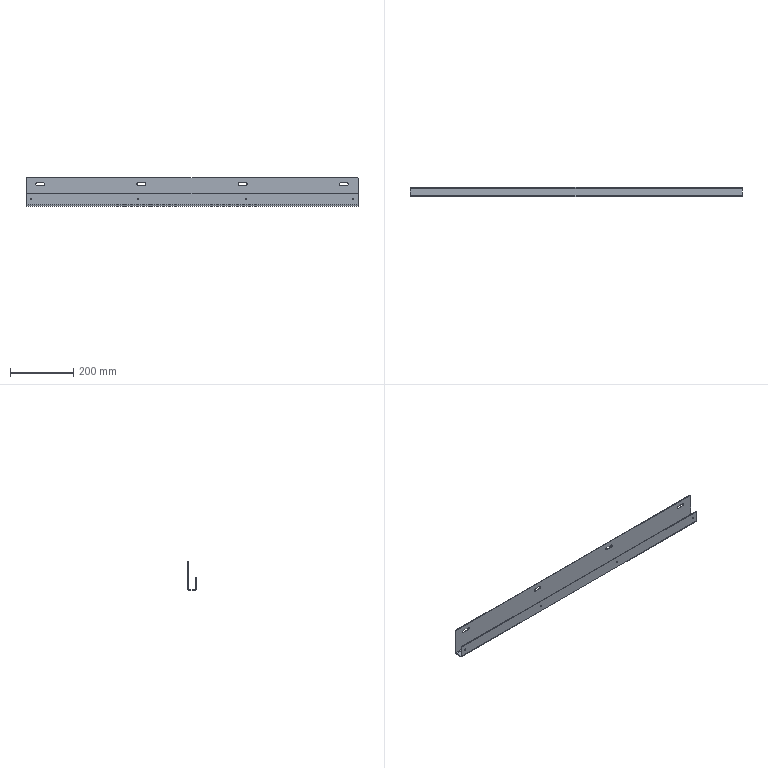Part | NX | features BREP 1 | 1 solid | 50 faces | box 1050 x 28.5 x 90 mm | volume 317181 mm3 | plane 30 | cylinder 20 | commonest cylinder face diameters 4.2 x8 8.2 x8 4 x2 8 x2
STEP:
#1=CARTESIAN_POINT('',(525.,-28.5,-52.));
#2=VERTEX_POINT('',#1);
#3=CARTESIAN_POINT('',(523.,-28.5,-50.));
#4=VERTEX_POINT('',#3);
#5=CARTESIAN_POINT('',(523.,-28.5,-50.));
#6=DIRECTION('',(-0.7071,0.,0.7071));
#7=VECTOR('',#6,1000.);
#8=LINE('',#5,#7);
#9=EDGE_CURVE('',#2,#4,#8,.T.);
#10=ORIENTED_EDGE('',*,*,#9,.F.);
#11=CARTESIAN_POINT('',(525.,-26.5,-52.));
#12=VERTEX_POINT('',#11);
#13=CARTESIAN_POINT('',(525.,-24.5,-52.));
#14=DIRECTION('',(0.,-1.,0.));
#15=VECTOR('',#14,1000.);
#16=LINE('',#13,#15);
#17=EDGE_CURVE('',#12,#2,#16,.T.);
#18=ORIENTED_EDGE('',*,*,#17,.F.);
#19=CARTESIAN_POINT('',(523.,-26.5,-50.));
#20=VERTEX_POINT('',#19);
#21=CARTESIAN_POINT('',(544.,-26.5,-71.));
#22=DIRECTION('',(0.7071,0.,-0.7071));
#23=VECTOR('',#22,1000.);
#24=LINE('',#21,#23);
#25=EDGE_CURVE('',#20,#12,#24,.T.);
#26=ORIENTED_EDGE('',*,*,#25,.F.);
#27=CARTESIAN_POINT('',(523.,-28.5,-50.));
#28=DIRECTION('',(0.,1.,0.));
#29=VECTOR('',#28,1000.);
#30=LINE('',#27,#29);
#31=EDGE_CURVE('',#4,#20,#30,.T.);
#32=ORIENTED_EDGE('',*,*,#31,.F.);
#33=EDGE_LOOP('',(#10,#18,#26,#32));
#34=FACE_BOUND('',#33,.T.);
#35=CARTESIAN_POINT('',(523.,-28.5,-50.));
#36=DIRECTION('',(-0.7071,0.,-0.7071));
#37=DIRECTION('',(0.,1.,0.));
#38=AXIS2_PLACEMENT_3D('',#35,#36,#37);
#39=PLANE('',#38);
#40=ADVANCED_FACE('',(#34),#39,.F.);
#41=CARTESIAN_POINT('',(525.,-2.,-2.));
#42=VERTEX_POINT('',#41);
#43=CARTESIAN_POINT('',(523.,-2.,0.));
#44=VERTEX_POINT('',#43);
#45=CARTESIAN_POINT('',(569.,-2.,-46.));
#46=DIRECTION('',(-0.7071,0.,0.7071));
#47=VECTOR('',#46,1000.);
#48=LINE('',#45,#47);
#49=EDGE_CURVE('',#42,#44,#48,.T.);
#50=ORIENTED_EDGE('',*,*,#49,.F.);
#51=CARTESIAN_POINT('',(525.,0.,-2.));
#52=VERTEX_POINT('',#51);
#53=CARTESIAN_POINT('',(525.,-4.,-2.));
#54=DIRECTION('',(0.,-1.,0.));
#55=VECTOR('',#54,1000.);
#56=LINE('',#53,#55);
#57=EDGE_CURVE('',#52,#42,#56,.T.);
#58=ORIENTED_EDGE('',*,*,#57,.F.);
#59=CARTESIAN_POINT('',(523.,0.,0.));
#60=VERTEX_POINT('',#59);
#61=CARTESIAN_POINT('',(523.,0.,0.));
#62=DIRECTION('',(0.7071,0.,-0.7071));
#63=VECTOR('',#62,1000.);
#64=LINE('',#61,#63);
#65=EDGE_CURVE('',#60,#52,#64,.T.);
#66=ORIENTED_EDGE('',*,*,#65,.F.);
#67=CARTESIAN_POINT('',(523.,-2.,0.));
#68=DIRECTION('',(0.,1.,0.));
#69=VECTOR('',#68,1000.);
#70=LINE('',#67,#69);
#71=EDGE_CURVE('',#44,#60,#70,.T.);
#72=ORIENTED_EDGE('',*,*,#71,.F.);
#73=EDGE_LOOP('',(#50,#58,#66,#72));
#74=FACE_BOUND('',#73,.T.);
#75=CARTESIAN_POINT('',(523.,-2.,0.));
#76=DIRECTION('',(-0.7071,0.,-0.7071));
#77=DIRECTION('',(0.,1.,0.));
#78=AXIS2_PLACEMENT_3D('',#75,#76,#77);
#79=PLANE('',#78);
#80=ADVANCED_FACE('',(#74),#79,.F.);
#81=CARTESIAN_POINT('',(-523.,-28.5,-50.));
#82=VERTEX_POINT('',#81);
#83=CARTESIAN_POINT('',(-525.,-28.5,-52.));
#84=VERTEX_POINT('',#83);
#85=CARTESIAN_POINT('',(-525.,-28.5,-52.));
#86=DIRECTION('',(-0.7071,0.,-0.7071));
#87=VECTOR('',#86,1000.);
#88=LINE('',#85,#87);
#89=EDGE_CURVE('',#82,#84,#88,.T.);
#90=ORIENTED_EDGE('',*,*,#89,.F.);
#91=CARTESIAN_POINT('',(-523.,-26.5,-50.));
#92=VERTEX_POINT('',#91);
#93=CARTESIAN_POINT('',(-523.,-28.5,-50.));
#94=DIRECTION('',(0.,-1.,0.));
#95=VECTOR('',#94,1000.);
#96=LINE('',#93,#95);
#97=EDGE_CURVE('',#92,#82,#96,.T.);
#98=ORIENTED_EDGE('',*,*,#97,.F.);
#99=CARTESIAN_POINT('',(-525.,-26.5,-52.));
#100=VERTEX_POINT('',#99);
#101=CARTESIAN_POINT('',(-19.,-26.5,454.));
#102=DIRECTION('',(0.7071,0.,0.7071));
#103=VECTOR('',#102,1000.);
#104=LINE('',#101,#103);
#105=EDGE_CURVE('',#100,#92,#104,.T.);
#106=ORIENTED_EDGE('',*,*,#105,.F.);
#107=CARTESIAN_POINT('',(-525.,-26.5,-52.));
#108=DIRECTION('',(0.,1.,0.));
#109=VECTOR('',#108,1000.);
#110=LINE('',#107,#109);
#111=EDGE_CURVE('',#84,#100,#110,.T.);
#112=ORIENTED_EDGE('',*,*,#111,.F.);
#113=EDGE_LOOP('',(#90,#98,#106,#112));
#114=FACE_BOUND('',#113,.T.);
#115=CARTESIAN_POINT('',(-525.,-4.,-52.));
#116=DIRECTION('',(-0.7071,0.,0.7071));
#117=DIRECTION('',(0.,-1.,0.));
#118=AXIS2_PLACEMENT_3D('',#115,#116,#117);
#119=PLANE('',#118);
#120=ADVANCED_FACE('',(#114),#119,.T.);
#121=CARTESIAN_POINT('',(-523.,-2.,0.));
#122=VERTEX_POINT('',#121);
#123=CARTESIAN_POINT('',(-525.,-2.,-2.));
#124=VERTEX_POINT('',#123);
#125=CARTESIAN_POINT('',(-44.,-2.,479.));
#126=DIRECTION('',(-0.7071,0.,-0.7071));
#127=VECTOR('',#126,1000.);
#128=LINE('',#125,#127);
#129=EDGE_CURVE('',#122,#124,#128,.T.);
#130=ORIENTED_EDGE('',*,*,#129,.F.);
#131=CARTESIAN_POINT('',(-523.,0.,0.));
#132=VERTEX_POINT('',#131);
#133=CARTESIAN_POINT('',(-523.,-2.,0.));
#134=DIRECTION('',(0.,-1.,0.));
#135=VECTOR('',#134,1000.);
#136=LINE('',#133,#135);
#137=EDGE_CURVE('',#132,#122,#136,.T.);
#138=ORIENTED_EDGE('',*,*,#137,.F.);
#139=CARTESIAN_POINT('',(-525.,0.,-2.));
#140=VERTEX_POINT('',#139);
#141=CARTESIAN_POINT('',(-525.,0.,-2.));
#142=DIRECTION('',(0.7071,0.,0.7071));
#143=VECTOR('',#142,1000.);
#144=LINE('',#141,#143);
#145=EDGE_CURVE('',#140,#132,#144,.T.);
#146=ORIENTED_EDGE('',*,*,#145,.F.);
#147=CARTESIAN_POINT('',(-525.,-4.,-2.));
#148=DIRECTION('',(0.,1.,0.));
#149=VECTOR('',#148,1000.);
#150=LINE('',#147,#149);
#151=EDGE_CURVE('',#124,#140,#150,.T.);
#152=ORIENTED_EDGE('',*,*,#151,.F.);
#153=EDGE_LOOP('',(#130,#138,#146,#152));
#154=FACE_BOUND('',#153,.T.);
#155=CARTESIAN_POINT('',(-525.,-4.,-2.));
#156=DIRECTION('',(0.7071,0.,-0.7071));
#157=DIRECTION('',(0.,1.,0.));
#158=AXIS2_PLACEMENT_3D('',#155,#156,#157);
#159=PLANE('',#158);
#160=ADVANCED_FACE('',(#154),#159,.F.);
#161=CARTESIAN_POINT('',(510.,-26.5,-65.9));
#162=VERTEX_POINT('',#161);
#163=CARTESIAN_POINT('',(510.,-28.5,-65.9));
#164=VERTEX_POINT('',#163);
#165=CARTESIAN_POINT('',(510.,-28.5,-65.9));
#166=DIRECTION('',(0.,-1.,0.));
#167=VECTOR('',#166,1000.);
#168=LINE('',#165,#167);
#169=EDGE_CURVE('',#162,#164,#168,.T.);
#170=ORIENTED_EDGE('',*,*,#169,.F.);
#171=CARTESIAN_POINT('',(510.,-26.5,-70.1));
#172=VERTEX_POINT('',#171);
#173=CARTESIAN_POINT('',(510.,-26.5,-68.));
#174=DIRECTION('',(0.,1.,0.));
#175=DIRECTION('',(0.,0.,1.));
#176=AXIS2_PLACEMENT_3D('',#173,#174,#175);
#177=CIRCLE('',#176,2.1);
#178=EDGE_CURVE('',#162,#172,#177,.T.);
#179=ORIENTED_EDGE('',*,*,#178,.T.);
#180=CARTESIAN_POINT('',(510.,-28.5,-70.1));
#181=VERTEX_POINT('',#180);
#182=CARTESIAN_POINT('',(510.,-28.5,-70.1));
#183=DIRECTION('',(0.,-1.,0.));
#184=VECTOR('',#183,1000.);
#185=LINE('',#182,#184);
#186=EDGE_CURVE('',#172,#181,#185,.T.);
#187=ORIENTED_EDGE('',*,*,#186,.T.);
#188=CARTESIAN_POINT('',(510.,-28.5,-68.));
#189=DIRECTION('',(0.,-1.,0.));
#190=DIRECTION('',(0.,0.,-1.));
#191=AXIS2_PLACEMENT_3D('',#188,#189,#190);
#192=CIRCLE('',#191,2.1);
#193=EDGE_CURVE('',#181,#164,#192,.T.);
#194=ORIENTED_EDGE('',*,*,#193,.T.);
#195=EDGE_LOOP('',(#170,#179,#187,#194));
#196=FACE_BOUND('',#195,.T.);
#197=CARTESIAN_POINT('',(510.,-28.5,-68.));
#198=DIRECTION('',(0.,-1.,0.));
#199=DIRECTION('',(0.,0.,-1.));
#200=AXIS2_PLACEMENT_3D('',#197,#198,#199);
#201=CYLINDRICAL_SURFACE('',#200,2.1);
#202=ADVANCED_FACE('',(#196),#201,.F.);
#203=CARTESIAN_POINT('',(170.,-26.5,-65.9));
#204=VERTEX_POINT('',#203);
#205=CARTESIAN_POINT('',(170.,-28.5,-65.9));
#206=VERTEX_POINT('',#205);
#207=CARTESIAN_POINT('',(170.,-28.5,-65.9));
#208=DIRECTION('',(0.,-1.,0.));
#209=VECTOR('',#208,1000.);
#210=LINE('',#207,#209);
#211=EDGE_CURVE('',#204,#206,#210,.T.);
#212=ORIENTED_EDGE('',*,*,#211,.F.);
#213=CARTESIAN_POINT('',(170.,-26.5,-70.1));
#214=VERTEX_POINT('',#213);
#215=CARTESIAN_POINT('',(170.,-26.5,-68.));
#216=DIRECTION('',(0.,1.,0.));
#217=DIRECTION('',(0.,0.,1.));
#218=AXIS2_PLACEMENT_3D('',#215,#216,#217);
#219=CIRCLE('',#218,2.1);
#220=EDGE_CURVE('',#204,#214,#219,.T.);
#221=ORIENTED_EDGE('',*,*,#220,.T.);
#222=CARTESIAN_POINT('',(170.,-28.5,-70.1));
#223=VERTEX_POINT('',#222);
#224=CARTESIAN_POINT('',(170.,-28.5,-70.1));
#225=DIRECTION('',(0.,-1.,0.));
#226=VECTOR('',#225,1000.);
#227=LINE('',#224,#226);
#228=EDGE_CURVE('',#214,#223,#227,.T.);
#229=ORIENTED_EDGE('',*,*,#228,.T.);
#230=CARTESIAN_POINT('',(170.,-28.5,-68.));
#231=DIRECTION('',(0.,-1.,0.));
#232=DIRECTION('',(0.,0.,-1.));
#233=AXIS2_PLACEMENT_3D('',#230,#231,#232);
#234=CIRCLE('',#233,2.1);
#235=EDGE_CURVE('',#223,#206,#234,.T.);
#236=ORIENTED_EDGE('',*,*,#235,.T.);
#237=EDGE_LOOP('',(#212,#221,#229,#236));
#238=FACE_BOUND('',#237,.T.);
#239=CARTESIAN_POINT('',(170.,-28.5,-68.));
#240=DIRECTION('',(0.,-1.,0.));
#241=DIRECTION('',(0.,0.,-1.));
#242=AXIS2_PLACEMENT_3D('',#239,#240,#241);
#243=CYLINDRICAL_SURFACE('',#242,2.1);
#244=ADVANCED_FACE('',(#238),#243,.F.);
#245=CARTESIAN_POINT('',(-170.,-26.5,-65.9));
#246=VERTEX_POINT('',#245);
#247=CARTESIAN_POINT('',(-170.,-28.5,-65.9));
#248=VERTEX_POINT('',#247);
#249=CARTESIAN_POINT('',(-170.,-28.5,-65.9));
#250=DIRECTION('',(0.,-1.,0.));
#251=VECTOR('',#250,1000.);
#252=LINE('',#249,#251);
#253=EDGE_CURVE('',#246,#248,#252,.T.);
#254=ORIENTED_EDGE('',*,*,#253,.F.);
#255=CARTESIAN_POINT('',(-170.,-26.5,-70.1));
#256=VERTEX_POINT('',#255);
#257=CARTESIAN_POINT('',(-170.,-26.5,-68.));
#258=DIRECTION('',(0.,1.,0.));
#259=DIRECTION('',(0.,0.,1.));
#260=AXIS2_PLACEMENT_3D('',#257,#258,#259);
#261=CIRCLE('',#260,2.1);
#262=EDGE_CURVE('',#246,#256,#261,.T.);
#263=ORIENTED_EDGE('',*,*,#262,.T.);
#264=CARTESIAN_POINT('',(-170.,-28.5,-70.1));
#265=VERTEX_POINT('',#264);
#266=CARTESIAN_POINT('',(-170.,-28.5,-70.1));
#267=DIRECTION('',(0.,-1.,0.));
#268=VECTOR('',#267,1000.);
#269=LINE('',#266,#268);
#270=EDGE_CURVE('',#256,#265,#269,.T.);
#271=ORIENTED_EDGE('',*,*,#270,.T.);
#272=CARTESIAN_POINT('',(-170.,-28.5,-68.));
#273=DIRECTION('',(0.,-1.,0.));
#274=DIRECTION('',(0.,0.,-1.));
#275=AXIS2_PLACEMENT_3D('',#272,#273,#274);
#276=CIRCLE('',#275,2.1);
#277=EDGE_CURVE('',#265,#248,#276,.T.);
#278=ORIENTED_EDGE('',*,*,#277,.T.);
#279=EDGE_LOOP('',(#254,#263,#271,#278));
#280=FACE_BOUND('',#279,.T.);
#281=CARTESIAN_POINT('',(-170.,-28.5,-68.));
#282=DIRECTION('',(0.,-1.,0.));
#283=DIRECTION('',(0.,0.,-1.));
#284=AXIS2_PLACEMENT_3D('',#281,#282,#283);
#285=CYLINDRICAL_SURFACE('',#284,2.1);
#286=ADVANCED_FACE('',(#280),#285,.F.);
#287=CARTESIAN_POINT('',(-510.,-26.5,-65.9));
#288=VERTEX_POINT('',#287);
#289=CARTESIAN_POINT('',(-510.,-28.5,-65.9));
#290=VERTEX_POINT('',#289);
#291=CARTESIAN_POINT('',(-510.,-28.5,-65.9));
#292=DIRECTION('',(0.,-1.,0.));
#293=VECTOR('',#292,1000.);
#294=LINE('',#291,#293);
#295=EDGE_CURVE('',#288,#290,#294,.T.);
#296=ORIENTED_EDGE('',*,*,#295,.F.);
#297=CARTESIAN_POINT('',(-510.,-26.5,-70.1));
#298=VERTEX_POINT('',#297);
#299=CARTESIAN_POINT('',(-510.,-26.5,-68.));
#300=DIRECTION('',(0.,1.,0.));
#301=DIRECTION('',(0.,0.,1.));
#302=AXIS2_PLACEMENT_3D('',#299,#300,#301);
#303=CIRCLE('',#302,2.1);
#304=EDGE_CURVE('',#288,#298,#303,.T.);
#305=ORIENTED_EDGE('',*,*,#304,.T.);
#306=CARTESIAN_POINT('',(-510.,-28.5,-70.1));
#307=VERTEX_POINT('',#306);
#308=CARTESIAN_POINT('',(-510.,-28.5,-70.1));
#309=DIRECTION('',(0.,-1.,0.));
#310=VECTOR('',#309,1000.);
#311=LINE('',#308,#310);
#312=EDGE_CURVE('',#298,#307,#311,.T.);
#313=ORIENTED_EDGE('',*,*,#312,.T.);
#314=CARTESIAN_POINT('',(-510.,-28.5,-68.));
#315=DIRECTION('',(0.,-1.,0.));
#316=DIRECTION('',(0.,0.,-1.));
#317=AXIS2_PLACEMENT_3D('',#314,#315,#316);
#318=CIRCLE('',#317,2.1);
#319=EDGE_CURVE('',#307,#290,#318,.T.);
#320=ORIENTED_EDGE('',*,*,#319,.T.);
#321=EDGE_LOOP('',(#296,#305,#313,#320));
#322=FACE_BOUND('',#321,.T.);
#323=CARTESIAN_POINT('',(-510.,-28.5,-68.));
#324=DIRECTION('',(0.,-1.,0.));
#325=DIRECTION('',(0.,0.,-1.));
#326=AXIS2_PLACEMENT_3D('',#323,#324,#325);
#327=CYLINDRICAL_SURFACE('',#326,2.1);
#328=ADVANCED_FACE('',(#322),#327,.F.);
#329=CARTESIAN_POINT('',(-470.,-2.,-15.9));
#330=VERTEX_POINT('',#329);
#331=CARTESIAN_POINT('',(-490.,-2.,-15.9));
#332=VERTEX_POINT('',#331);
#333=CARTESIAN_POINT('',(525.,-2.,-15.9));
#334=DIRECTION('',(-1.,0.,0.));
#335=VECTOR('',#334,1000.);
#336=LINE('',#333,#335);
#337=EDGE_CURVE('',#330,#332,#336,.T.);
#338=ORIENTED_EDGE('',*,*,#337,.T.);
#339=CARTESIAN_POINT('',(-490.,0.,-15.9));
#340=VERTEX_POINT('',#339);
#341=CARTESIAN_POINT('',(-490.,0.,-15.9));
#342=DIRECTION('',(0.,1.,0.));
#343=VECTOR('',#342,1000.);
#344=LINE('',#341,#343);
#345=EDGE_CURVE('',#332,#340,#344,.T.);
#346=ORIENTED_EDGE('',*,*,#345,.T.);
#347=CARTESIAN_POINT('',(-470.,0.,-15.9));
#348=VERTEX_POINT('',#347);
#349=CARTESIAN_POINT('',(-490.,0.,-15.9));
#350=DIRECTION('',(1.,0.,0.));
#351=VECTOR('',#350,1000.);
#352=LINE('',#349,#351);
#353=EDGE_CURVE('',#340,#348,#352,.T.);
#354=ORIENTED_EDGE('',*,*,#353,.T.);
#355=CARTESIAN_POINT('',(-470.,0.,-15.9));
#356=DIRECTION('',(0.,-1.,0.));
#357=VECTOR('',#356,1000.);
#358=LINE('',#355,#357);
#359=EDGE_CURVE('',#348,#330,#358,.T.);
#360=ORIENTED_EDGE('',*,*,#359,.T.);
#361=EDGE_LOOP('',(#338,#346,#354,#360));
#362=FACE_BOUND('',#361,.T.);
#363=CARTESIAN_POINT('',(-490.,0.,-15.9));
#364=DIRECTION('',(0.,0.,1.));
#365=DIRECTION('',(1.,0.,0.));
#366=AXIS2_PLACEMENT_3D('',#363,#364,#365);
#367=PLANE('',#366);
#368=ADVANCED_FACE('',(#362),#367,.F.);
#369=CARTESIAN_POINT('',(-490.,-2.,-24.1));
#370=VERTEX_POINT('',#369);
#371=CARTESIAN_POINT('',(-470.,-2.,-24.1));
#372=VERTEX_POINT('',#371);
#373=CARTESIAN_POINT('',(525.,-2.,-24.1));
#374=DIRECTION('',(1.,0.,0.));
#375=VECTOR('',#374,1000.);
#376=LINE('',#373,#375);
#377=EDGE_CURVE('',#370,#372,#376,.T.);
#378=ORIENTED_EDGE('',*,*,#377,.T.);
#379=CARTESIAN_POINT('',(-470.,0.,-24.1));
#380=VERTEX_POINT('',#379);
#381=CARTESIAN_POINT('',(-470.,0.,-24.1));
#382=DIRECTION('',(0.,1.,0.));
#383=VECTOR('',#382,1000.);
#384=LINE('',#381,#383);
#385=EDGE_CURVE('',#372,#380,#384,.T.);
#386=ORIENTED_EDGE('',*,*,#385,.T.);
#387=CARTESIAN_POINT('',(-490.,0.,-24.1));
#388=VERTEX_POINT('',#387);
#389=CARTESIAN_POINT('',(-490.,0.,-24.1));
#390=DIRECTION('',(1.,0.,0.));
#391=VECTOR('',#390,1000.);
#392=LINE('',#389,#391);
#393=EDGE_CURVE('',#388,#380,#392,.T.);
#394=ORIENTED_EDGE('',*,*,#393,.F.);
#395=CARTESIAN_POINT('',(-490.,0.,-24.1));
#396=DIRECTION('',(0.,-1.,0.));
#397=VECTOR('',#396,1000.);
#398=LINE('',#395,#397);
#399=EDGE_CURVE('',#388,#370,#398,.T.);
#400=ORIENTED_EDGE('',*,*,#399,.T.);
#401=EDGE_LOOP('',(#378,#386,#394,#400));
#402=FACE_BOUND('',#401,.T.);
#403=CARTESIAN_POINT('',(-490.,0.,-24.1));
#404=DIRECTION('',(0.,0.,-1.));
#405=DIRECTION('',(-1.,0.,0.));
#406=AXIS2_PLACEMENT_3D('',#403,#404,#405);
#407=PLANE('',#406);
#408=ADVANCED_FACE('',(#402),#407,.F.);
#409=CARTESIAN_POINT('',(-490.,-2.,-20.));
#410=DIRECTION('',(0.,-1.,0.));
#411=DIRECTION('',(0.,0.,-1.));
#412=AXIS2_PLACEMENT_3D('',#409,#410,#411);
#413=CIRCLE('',#412,4.1);
#414=EDGE_CURVE('',#332,#370,#413,.T.);
#415=ORIENTED_EDGE('',*,*,#414,.T.);
#416=ORIENTED_EDGE('',*,*,#399,.F.);
#417=CARTESIAN_POINT('',(-490.,0.,-20.));
#418=DIRECTION('',(0.,1.,0.));
#419=DIRECTION('',(0.,0.,1.));
#420=AXIS2_PLACEMENT_3D('',#417,#418,#419);
#421=CIRCLE('',#420,4.1);
#422=EDGE_CURVE('',#388,#340,#421,.T.);
#423=ORIENTED_EDGE('',*,*,#422,.T.);
#424=ORIENTED_EDGE('',*,*,#345,.F.);
#425=EDGE_LOOP('',(#415,#416,#423,#424));
#426=FACE_BOUND('',#425,.T.);
#427=CARTESIAN_POINT('',(-490.,0.,-20.));
#428=DIRECTION('',(0.,1.,0.));
#429=DIRECTION('',(0.,0.,1.));
#430=AXIS2_PLACEMENT_3D('',#427,#428,#429);
#431=CYLINDRICAL_SURFACE('',#430,4.1);
#432=ADVANCED_FACE('',(#426),#431,.F.);
#433=CARTESIAN_POINT('',(-470.,-2.,-20.));
#434=DIRECTION('',(0.,-1.,0.));
#435=DIRECTION('',(0.,0.,-1.));
#436=AXIS2_PLACEMENT_3D('',#433,#434,#435);
#437=CIRCLE('',#436,4.1);
#438=EDGE_CURVE('',#372,#330,#437,.T.);
#439=ORIENTED_EDGE('',*,*,#438,.T.);
#440=ORIENTED_EDGE('',*,*,#359,.F.);
#441=CARTESIAN_POINT('',(-470.,0.,-20.));
#442=DIRECTION('',(0.,1.,0.));
#443=DIRECTION('',(0.,0.,1.));
#444=AXIS2_PLACEMENT_3D('',#441,#442,#443);
#445=CIRCLE('',#444,4.1);
#446=EDGE_CURVE('',#348,#380,#445,.T.);
#447=ORIENTED_EDGE('',*,*,#446,.T.);
#448=ORIENTED_EDGE('',*,*,#385,.F.);
#449=EDGE_LOOP('',(#439,#440,#447,#448));
#450=FACE_BOUND('',#449,.T.);
#451=CARTESIAN_POINT('',(-470.,0.,-20.));
#452=DIRECTION('',(0.,1.,0.));
#453=DIRECTION('',(0.,0.,1.));
#454=AXIS2_PLACEMENT_3D('',#451,#452,#453);
#455=CYLINDRICAL_SURFACE('',#454,4.1);
#456=ADVANCED_FACE('',(#450),#455,.F.);
#457=CARTESIAN_POINT('',(-150.,-2.,-15.9));
#458=VERTEX_POINT('',#457);
#459=CARTESIAN_POINT('',(-170.,-2.,-15.9));
#460=VERTEX_POINT('',#459);
#461=CARTESIAN_POINT('',(525.,-2.,-15.9));
#462=DIRECTION('',(-1.,0.,0.));
#463=VECTOR('',#462,1000.);
#464=LINE('',#461,#463);
#465=EDGE_CURVE('',#458,#460,#464,.T.);
#466=ORIENTED_EDGE('',*,*,#465,.T.);
#467=CARTESIAN_POINT('',(-170.,0.,-15.9));
#468=VERTEX_POINT('',#467);
#469=CARTESIAN_POINT('',(-170.,0.,-15.9));
#470=DIRECTION('',(0.,1.,0.));
#471=VECTOR('',#470,1000.);
#472=LINE('',#469,#471);
#473=EDGE_CURVE('',#460,#468,#472,.T.);
#474=ORIENTED_EDGE('',*,*,#473,.T.);
#475=CARTESIAN_POINT('',(-150.,0.,-15.9));
#476=VERTEX_POINT('',#475);
#477=CARTESIAN_POINT('',(-170.,0.,-15.9));
#478=DIRECTION('',(1.,0.,0.));
#479=VECTOR('',#478,1000.);
#480=LINE('',#477,#479);
#481=EDGE_CURVE('',#468,#476,#480,.T.);
#482=ORIENTED_EDGE('',*,*,#481,.T.);
#483=CARTESIAN_POINT('',(-150.,0.,-15.9));
#484=DIRECTION('',(0.,-1.,0.));
#485=VECTOR('',#484,1000.);
#486=LINE('',#483,#485);
#487=EDGE_CURVE('',#476,#458,#486,.T.);
#488=ORIENTED_EDGE('',*,*,#487,.T.);
#489=EDGE_LOOP('',(#466,#474,#482,#488));
#490=FACE_BOUND('',#489,.T.);
#491=CARTESIAN_POINT('',(-170.,0.,-15.9));
#492=DIRECTION('',(0.,0.,1.));
#493=DIRECTION('',(1.,0.,0.));
#494=AXIS2_PLACEMENT_3D('',#491,#492,#493);
#495=PLANE('',#494);
#496=ADVANCED_FACE('',(#490),#495,.F.);
#497=CARTESIAN_POINT('',(-170.,-2.,-24.1));
#498=VERTEX_POINT('',#497);
#499=CARTESIAN_POINT('',(-150.,-2.,-24.1));
#500=VERTEX_POINT('',#499);
#501=CARTESIAN_POINT('',(525.,-2.,-24.1));
#502=DIRECTION('',(1.,0.,0.));
#503=VECTOR('',#502,1000.);
#504=LINE('',#501,#503);
#505=EDGE_CURVE('',#498,#500,#504,.T.);
#506=ORIENTED_EDGE('',*,*,#505,.T.);
#507=CARTESIAN_POINT('',(-150.,0.,-24.1));
#508=VERTEX_POINT('',#507);
#509=CARTESIAN_POINT('',(-150.,0.,-24.1));
#510=DIRECTION('',(0.,1.,0.));
#511=VECTOR('',#510,1000.);
#512=LINE('',#509,#511);
#513=EDGE_CURVE('',#500,#508,#512,.T.);
#514=ORIENTED_EDGE('',*,*,#513,.T.);
#515=CARTESIAN_POINT('',(-170.,0.,-24.1));
#516=VERTEX_POINT('',#515);
#517=CARTESIAN_POINT('',(-170.,0.,-24.1));
#518=DIRECTION('',(1.,0.,0.));
#519=VECTOR('',#518,1000.);
#520=LINE('',#517,#519);
#521=EDGE_CURVE('',#516,#508,#520,.T.);
#522=ORIENTED_EDGE('',*,*,#521,.F.);
#523=CARTESIAN_POINT('',(-170.,0.,-24.1));
#524=DIRECTION('',(0.,-1.,0.));
#525=VECTOR('',#524,1000.);
#526=LINE('',#523,#525);
#527=EDGE_CURVE('',#516,#498,#526,.T.);
#528=ORIENTED_EDGE('',*,*,#527,.T.);
#529=EDGE_LOOP('',(#506,#514,#522,#528));
#530=FACE_BOUND('',#529,.T.);
#531=CARTESIAN_POINT('',(-170.,0.,-24.1));
#532=DIRECTION('',(0.,0.,-1.));
#533=DIRECTION('',(-1.,0.,0.));
#534=AXIS2_PLACEMENT_3D('',#531,#532,#533);
#535=PLANE('',#534);
#536=ADVANCED_FACE('',(#530),#535,.F.);
#537=CARTESIAN_POINT('',(-170.,-2.,-20.));
#538=DIRECTION('',(0.,-1.,0.));
#539=DIRECTION('',(0.,0.,-1.));
#540=AXIS2_PLACEMENT_3D('',#537,#538,#539);
#541=CIRCLE('',#540,4.1);
#542=EDGE_CURVE('',#460,#498,#541,.T.);
#543=ORIENTED_EDGE('',*,*,#542,.T.);
#544=ORIENTED_EDGE('',*,*,#527,.F.);
#545=CARTESIAN_POINT('',(-170.,0.,-20.));
#546=DIRECTION('',(0.,1.,0.));
#547=DIRECTION('',(0.,0.,1.));
#548=AXIS2_PLACEMENT_3D('',#545,#546,#547);
#549=CIRCLE('',#548,4.1);
#550=EDGE_CURVE('',#516,#468,#549,.T.);
#551=ORIENTED_EDGE('',*,*,#550,.T.);
#552=ORIENTED_EDGE('',*,*,#473,.F.);
#553=EDGE_LOOP('',(#543,#544,#551,#552));
#554=FACE_BOUND('',#553,.T.);
#555=CARTESIAN_POINT('',(-170.,0.,-20.));
#556=DIRECTION('',(0.,1.,0.));
#557=DIRECTION('',(0.,0.,1.));
#558=AXIS2_PLACEMENT_3D('',#555,#556,#557);
#559=CYLINDRICAL_SURFACE('',#558,4.1);
#560=ADVANCED_FACE('',(#554),#559,.F.);
#561=CARTESIAN_POINT('',(-150.,-2.,-20.));
#562=DIRECTION('',(0.,-1.,0.));
#563=DIRECTION('',(0.,0.,-1.));
#564=AXIS2_PLACEMENT_3D('',#561,#562,#563);
#565=CIRCLE('',#564,4.1);
#566=EDGE_CURVE('',#500,#458,#565,.T.);
#567=ORIENTED_EDGE('',*,*,#566,.T.);
#568=ORIENTED_EDGE('',*,*,#487,.F.);
#569=CARTESIAN_POINT('',(-150.,0.,-20.));
#570=DIRECTION('',(0.,1.,0.));
#571=DIRECTION('',(0.,0.,1.));
#572=AXIS2_PLACEMENT_3D('',#569,#570,#571);
#573=CIRCLE('',#572,4.1);
#574=EDGE_CURVE('',#476,#508,#573,.T.);
#575=ORIENTED_EDGE('',*,*,#574,.T.);
#576=ORIENTED_EDGE('',*,*,#513,.F.);
#577=EDGE_LOOP('',(#567,#568,#575,#576));
#578=FACE_BOUND('',#577,.T.);
#579=CARTESIAN_POINT('',(-150.,0.,-20.));
#580=DIRECTION('',(0.,1.,0.));
#581=DIRECTION('',(0.,0.,1.));
#582=AXIS2_PLACEMENT_3D('',#579,#580,#581);
#583=CYLINDRICAL_SURFACE('',#582,4.1);
#584=ADVANCED_FACE('',(#578),#583,.F.);
#585=CARTESIAN_POINT('',(170.,-2.,-15.9));
#586=VERTEX_POINT('',#585);
#587=CARTESIAN_POINT('',(150.,-2.,-15.9));
#588=VERTEX_POINT('',#587);
#589=CARTESIAN_POINT('',(525.,-2.,-15.9));
#590=DIRECTION('',(-1.,0.,0.));
#591=VECTOR('',#590,1000.);
#592=LINE('',#589,#591);
#593=EDGE_CURVE('',#586,#588,#592,.T.);
#594=ORIENTED_EDGE('',*,*,#593,.T.);
#595=CARTESIAN_POINT('',(150.,0.,-15.9));
#596=VERTEX_POINT('',#595);
#597=CARTESIAN_POINT('',(150.,0.,-15.9));
#598=DIRECTION('',(0.,1.,0.));
#599=VECTOR('',#598,1000.);
#600=LINE('',#597,#599);
#601=EDGE_CURVE('',#588,#596,#600,.T.);
#602=ORIENTED_EDGE('',*,*,#601,.T.);
#603=CARTESIAN_POINT('',(170.,0.,-15.9));
#604=VERTEX_POINT('',#603);
#605=CARTESIAN_POINT('',(150.,0.,-15.9));
#606=DIRECTION('',(1.,0.,0.));
#607=VECTOR('',#606,1000.);
#608=LINE('',#605,#607);
#609=EDGE_CURVE('',#596,#604,#608,.T.);
#610=ORIENTED_EDGE('',*,*,#609,.T.);
#611=CARTESIAN_POINT('',(170.,0.,-15.9));
#612=DIRECTION('',(0.,-1.,0.));
#613=VECTOR('',#612,1000.);
#614=LINE('',#611,#613);
#615=EDGE_CURVE('',#604,#586,#614,.T.);
#616=ORIENTED_EDGE('',*,*,#615,.T.);
#617=EDGE_LOOP('',(#594,#602,#610,#616));
#618=FACE_BOUND('',#617,.T.);
#619=CARTESIAN_POINT('',(150.,0.,-15.9));
#620=DIRECTION('',(0.,0.,1.));
#621=DIRECTION('',(0.,-1.,0.));
#622=AXIS2_PLACEMENT_3D('',#619,#620,#621);
#623=PLANE('',#622);
#624=ADVANCED_FACE('',(#618),#623,.F.);
#625=CARTESIAN_POINT('',(150.,-2.,-24.1));
#626=VERTEX_POINT('',#625);
#627=CARTESIAN_POINT('',(170.,-2.,-24.1));
#628=VERTEX_POINT('',#627);
#629=CARTESIAN_POINT('',(525.,-2.,-24.1));
#630=DIRECTION('',(1.,0.,0.));
#631=VECTOR('',#630,1000.);
#632=LINE('',#629,#631);
#633=EDGE_CURVE('',#626,#628,#632,.T.);
#634=ORIENTED_EDGE('',*,*,#633,.T.);
#635=CARTESIAN_POINT('',(170.,0.,-24.1));
#636=VERTEX_POINT('',#635);
#637=CARTESIAN_POINT('',(170.,0.,-24.1));
#638=DIRECTION('',(0.,1.,0.));
#639=VECTOR('',#638,1000.);
#640=LINE('',#637,#639);
#641=EDGE_CURVE('',#628,#636,#640,.T.);
#642=ORIENTED_EDGE('',*,*,#641,.T.);
#643=CARTESIAN_POINT('',(150.,0.,-24.1));
#644=VERTEX_POINT('',#643);
#645=CARTESIAN_POINT('',(150.,0.,-24.1));
#646=DIRECTION('',(1.,0.,0.));
#647=VECTOR('',#646,1000.);
#648=LINE('',#645,#647);
#649=EDGE_CURVE('',#644,#636,#648,.T.);
#650=ORIENTED_EDGE('',*,*,#649,.F.);
#651=CARTESIAN_POINT('',(150.,0.,-24.1));
#652=DIRECTION('',(0.,-1.,0.));
#653=VECTOR('',#652,1000.);
#654=LINE('',#651,#653);
#655=EDGE_CURVE('',#644,#626,#654,.T.);
#656=ORIENTED_EDGE('',*,*,#655,.T.);
#657=EDGE_LOOP('',(#634,#642,#650,#656));
#658=FACE_BOUND('',#657,.T.);
#659=CARTESIAN_POINT('',(150.,0.,-24.1));
#660=DIRECTION('',(0.,0.,-1.));
#661=DIRECTION('',(0.,1.,0.));
#662=AXIS2_PLACEMENT_3D('',#659,#660,#661);
#663=PLANE('',#662);
#664=ADVANCED_FACE('',(#658),#663,.F.);
#665=CARTESIAN_POINT('',(150.,-2.,-20.));
#666=DIRECTION('',(0.,-1.,0.));
#667=DIRECTION('',(0.,0.,-1.));
#668=AXIS2_PLACEMENT_3D('',#665,#666,#667);
#669=CIRCLE('',#668,4.1);
#670=EDGE_CURVE('',#588,#626,#669,.T.);
#671=ORIENTED_EDGE('',*,*,#670,.T.);
#672=ORIENTED_EDGE('',*,*,#655,.F.);
#673=CARTESIAN_POINT('',(150.,0.,-20.));
#674=DIRECTION('',(0.,1.,0.));
#675=DIRECTION('',(0.,0.,1.));
#676=AXIS2_PLACEMENT_3D('',#673,#674,#675);
#677=CIRCLE('',#676,4.1);
#678=EDGE_CURVE('',#644,#596,#677,.T.);
#679=ORIENTED_EDGE('',*,*,#678,.T.);
#680=ORIENTED_EDGE('',*,*,#601,.F.);
#681=EDGE_LOOP('',(#671,#672,#679,#680));
#682=FACE_BOUND('',#681,.T.);
#683=CARTESIAN_POINT('',(150.,0.,-20.));
#684=DIRECTION('',(0.,1.,0.));
#685=DIRECTION('',(0.,0.,1.));
#686=AXIS2_PLACEMENT_3D('',#683,#684,#685);
#687=CYLINDRICAL_SURFACE('',#686,4.1);
#688=ADVANCED_FACE('',(#682),#687,.F.);
#689=CARTESIAN_POINT('',(170.,-2.,-20.));
#690=DIRECTION('',(0.,-1.,0.));
#691=DIRECTION('',(0.,0.,-1.));
#692=AXIS2_PLACEMENT_3D('',#689,#690,#691);
#693=CIRCLE('',#692,4.1);
#694=EDGE_CURVE('',#628,#586,#693,.T.);
#695=ORIENTED_EDGE('',*,*,#694,.T.);
#696=ORIENTED_EDGE('',*,*,#615,.F.);
#697=CARTESIAN_POINT('',(170.,0.,-20.));
#698=DIRECTION('',(0.,1.,0.));
#699=DIRECTION('',(0.,0.,1.));
#700=AXIS2_PLACEMENT_3D('',#697,#698,#699);
#701=CIRCLE('',#700,4.1);
#702=EDGE_CURVE('',#604,#636,#701,.T.);
#703=ORIENTED_EDGE('',*,*,#702,.T.);
#704=ORIENTED_EDGE('',*,*,#641,.F.);
#705=EDGE_LOOP('',(#695,#696,#703,#704));
#706=FACE_BOUND('',#705,.T.);
#707=CARTESIAN_POINT('',(170.,0.,-20.));
#708=DIRECTION('',(0.,1.,0.));
#709=DIRECTION('',(0.,0.,1.));
#710=AXIS2_PLACEMENT_3D('',#707,#708,#709);
#711=CYLINDRICAL_SURFACE('',#710,4.1);
#712=ADVANCED_FACE('',(#706),#711,.F.);
#713=CARTESIAN_POINT('',(490.,-2.,-15.9));
#714=VERTEX_POINT('',#713);
#715=CARTESIAN_POINT('',(470.,-2.,-15.9));
#716=VERTEX_POINT('',#715);
#717=CARTESIAN_POINT('',(525.,-2.,-15.9));
#718=DIRECTION('',(-1.,0.,0.));
#719=VECTOR('',#718,1000.);
#720=LINE('',#717,#719);
#721=EDGE_CURVE('',#714,#716,#720,.T.);
#722=ORIENTED_EDGE('',*,*,#721,.T.);
#723=CARTESIAN_POINT('',(470.,0.,-15.9));
#724=VERTEX_POINT('',#723);
#725=CARTESIAN_POINT('',(470.,0.,-15.9));
#726=DIRECTION('',(0.,1.,0.));
#727=VECTOR('',#726,1000.);
#728=LINE('',#725,#727);
#729=EDGE_CURVE('',#716,#724,#728,.T.);
#730=ORIENTED_EDGE('',*,*,#729,.T.);
#731=CARTESIAN_POINT('',(490.,0.,-15.9));
#732=VERTEX_POINT('',#731);
#733=CARTESIAN_POINT('',(470.,0.,-15.9));
#734=DIRECTION('',(1.,0.,0.));
#735=VECTOR('',#734,1000.);
#736=LINE('',#733,#735);
#737=EDGE_CURVE('',#724,#732,#736,.T.);
#738=ORIENTED_EDGE('',*,*,#737,.T.);
#739=CARTESIAN_POINT('',(490.,0.,-15.9));
#740=DIRECTION('',(0.,-1.,0.));
#741=VECTOR('',#740,1000.);
#742=LINE('',#739,#741);
#743=EDGE_CURVE('',#732,#714,#742,.T.);
#744=ORIENTED_EDGE('',*,*,#743,.T.);
#745=EDGE_LOOP('',(#722,#730,#738,#744));
#746=FACE_BOUND('',#745,.T.);
#747=CARTESIAN_POINT('',(470.,0.,-15.9));
#748=DIRECTION('',(0.,0.,1.));
#749=DIRECTION('',(1.,0.,0.));
#750=AXIS2_PLACEMENT_3D('',#747,#748,#749);
#751=PLANE('',#750);
#752=ADVANCED_FACE('',(#746),#751,.F.);
#753=CARTESIAN_POINT('',(470.,-2.,-24.1));
#754=VERTEX_POINT('',#753);
#755=CARTESIAN_POINT('',(490.,-2.,-24.1));
#756=VERTEX_POINT('',#755);
#757=CARTESIAN_POINT('',(525.,-2.,-24.1));
#758=DIRECTION('',(1.,0.,0.));
#759=VECTOR('',#758,1000.);
#760=LINE('',#757,#759);
#761=EDGE_CURVE('',#754,#756,#760,.T.);
#762=ORIENTED_EDGE('',*,*,#761,.T.);
#763=CARTESIAN_POINT('',(490.,0.,-24.1));
#764=VERTEX_POINT('',#763);
#765=CARTESIAN_POINT('',(490.,0.,-24.1));
#766=DIRECTION('',(0.,1.,0.));
#767=VECTOR('',#766,1000.);
#768=LINE('',#765,#767);
#769=EDGE_CURVE('',#756,#764,#768,.T.);
#770=ORIENTED_EDGE('',*,*,#769,.T.);
#771=CARTESIAN_POINT('',(470.,0.,-24.1));
#772=VERTEX_POINT('',#771);
#773=CARTESIAN_POINT('',(470.,0.,-24.1));
#774=DIRECTION('',(1.,0.,0.));
#775=VECTOR('',#774,1000.);
#776=LINE('',#773,#775);
#777=EDGE_CURVE('',#772,#764,#776,.T.);
#778=ORIENTED_EDGE('',*,*,#777,.F.);
#779=CARTESIAN_POINT('',(470.,0.,-24.1));
#780=DIRECTION('',(0.,-1.,0.));
#781=VECTOR('',#780,1000.);
#782=LINE('',#779,#781);
#783=EDGE_CURVE('',#772,#754,#782,.T.);
#784=ORIENTED_EDGE('',*,*,#783,.T.);
#785=EDGE_LOOP('',(#762,#770,#778,#784));
#786=FACE_BOUND('',#785,.T.);
#787=CARTESIAN_POINT('',(470.,0.,-24.1));
#788=DIRECTION('',(0.,0.,-1.));
#789=DIRECTION('',(-1.,0.,0.));
#790=AXIS2_PLACEMENT_3D('',#787,#788,#789);
#791=PLANE('',#790);
#792=ADVANCED_FACE('',(#786),#791,.F.);
#793=CARTESIAN_POINT('',(470.,-2.,-20.));
#794=DIRECTION('',(0.,-1.,0.));
#795=DIRECTION('',(0.,0.,-1.));
#796=AXIS2_PLACEMENT_3D('',#793,#794,#795);
#797=CIRCLE('',#796,4.1);
#798=EDGE_CURVE('',#716,#754,#797,.T.);
#799=ORIENTED_EDGE('',*,*,#798,.T.);
#800=ORIENTED_EDGE('',*,*,#783,.F.);
#801=CARTESIAN_POINT('',(470.,0.,-20.));
#802=DIRECTION('',(0.,1.,0.));
#803=DIRECTION('',(0.,0.,1.));
#804=AXIS2_PLACEMENT_3D('',#801,#802,#803);
#805=CIRCLE('',#804,4.1);
#806=EDGE_CURVE('',#772,#724,#805,.T.);
#807=ORIENTED_EDGE('',*,*,#806,.T.);
#808=ORIENTED_EDGE('',*,*,#729,.F.);
#809=EDGE_LOOP('',(#799,#800,#807,#808));
#810=FACE_BOUND('',#809,.T.);
#811=CARTESIAN_POINT('',(470.,0.,-20.));
#812=DIRECTION('',(0.,1.,0.));
#813=DIRECTION('',(0.,0.,1.));
#814=AXIS2_PLACEMENT_3D('',#811,#812,#813);
#815=CYLINDRICAL_SURFACE('',#814,4.1);
#816=ADVANCED_FACE('',(#810),#815,.F.);
#817=CARTESIAN_POINT('',(490.,-2.,-20.));
#818=DIRECTION('',(0.,-1.,0.));
#819=DIRECTION('',(0.,0.,-1.));
#820=AXIS2_PLACEMENT_3D('',#817,#818,#819);
#821=CIRCLE('',#820,4.1);
#822=EDGE_CURVE('',#756,#714,#821,.T.);
#823=ORIENTED_EDGE('',*,*,#822,.T.);
#824=ORIENTED_EDGE('',*,*,#743,.F.);
#825=CARTESIAN_POINT('',(490.,0.,-20.));
#826=DIRECTION('',(0.,1.,0.));
#827=DIRECTION('',(0.,0.,1.));
#828=AXIS2_PLACEMENT_3D('',#825,#826,#827);
#829=CIRCLE('',#828,4.1);
#830=EDGE_CURVE('',#732,#764,#829,.T.);
#831=ORIENTED_EDGE('',*,*,#830,.T.);
#832=ORIENTED_EDGE('',*,*,#769,.F.);
#833=EDGE_LOOP('',(#823,#824,#831,#832));
#834=FACE_BOUND('',#833,.T.);
#835=CARTESIAN_POINT('',(490.,0.,-20.));
#836=DIRECTION('',(0.,1.,0.));
#837=DIRECTION('',(0.,0.,1.));
#838=AXIS2_PLACEMENT_3D('',#835,#836,#837);
#839=CYLINDRICAL_SURFACE('',#838,4.1);
#840=ADVANCED_FACE('',(#834),#839,.F.);
#841=CARTESIAN_POINT('',(-525.,-28.5,-86.));
#842=VERTEX_POINT('',#841);
#843=CARTESIAN_POINT('',(-525.,-28.5,-90.));
#844=DIRECTION('',(0.,0.,-1.));
#845=VECTOR('',#844,1000.);
#846=LINE('',#843,#845);
#847=EDGE_CURVE('',#84,#842,#846,.T.);
#848=ORIENTED_EDGE('',*,*,#847,.F.);
#849=ORIENTED_EDGE('',*,*,#111,.T.);
#850=CARTESIAN_POINT('',(-525.,-26.5,-86.));
#851=VERTEX_POINT('',#850);
#852=CARTESIAN_POINT('',(-525.,-26.5,-90.));
#853=DIRECTION('',(0.,0.,-1.));
#854=VECTOR('',#853,1000.);
#855=LINE('',#852,#854);
#856=EDGE_CURVE('',#100,#851,#855,.T.);
#857=ORIENTED_EDGE('',*,*,#856,.T.);
#858=CARTESIAN_POINT('',(-525.,-26.5,-86.));
#859=DIRECTION('',(0.,-1.,0.));
#860=VECTOR('',#859,1000.);
#861=LINE('',#858,#860);
#862=EDGE_CURVE('',#851,#842,#861,.T.);
#863=ORIENTED_EDGE('',*,*,#862,.T.);
#864=EDGE_LOOP('',(#848,#849,#857,#863));
#865=FACE_BOUND('',#864,.T.);
#866=CARTESIAN_POINT('',(-525.,-4.,-86.));
#867=DIRECTION('',(1.,0.,0.));
#868=DIRECTION('',(0.,0.,-1.));
#869=AXIS2_PLACEMENT_3D('',#866,#867,#868);
#870=PLANE('',#869);
#871=ADVANCED_FACE('',(#865),#870,.F.);
#872=CARTESIAN_POINT('',(525.,0.,-86.));
#873=VERTEX_POINT('',#872);
#874=CARTESIAN_POINT('',(525.,0.,-90.));
#875=DIRECTION('',(0.,0.,1.));
#876=VECTOR('',#875,1000.);
#877=LINE('',#874,#876);
#878=EDGE_CURVE('',#873,#52,#877,.T.);
#879=ORIENTED_EDGE('',*,*,#878,.T.);
#880=ORIENTED_EDGE('',*,*,#57,.T.);
#881=CARTESIAN_POINT('',(525.,-2.,-86.));
#882=VERTEX_POINT('',#881);
#883=CARTESIAN_POINT('',(525.,-2.,-90.));
#884=DIRECTION('',(0.,0.,1.));
#885=VECTOR('',#884,1000.);
#886=LINE('',#883,#885);
#887=EDGE_CURVE('',#882,#42,#886,.T.);
#888=ORIENTED_EDGE('',*,*,#887,.F.);
#889=CARTESIAN_POINT('',(525.,-2.,-86.));
#890=DIRECTION('',(0.,1.,0.));
#891=VECTOR('',#890,1000.);
#892=LINE('',#889,#891);
#893=EDGE_CURVE('',#882,#873,#892,.T.);
#894=ORIENTED_EDGE('',*,*,#893,.T.);
#895=EDGE_LOOP('',(#879,#880,#888,#894));
#896=FACE_BOUND('',#895,.T.);
#897=CARTESIAN_POINT('',(525.,-4.,-86.));
#898=DIRECTION('',(1.,0.,0.));
#899=DIRECTION('',(0.,0.,-1.));
#900=AXIS2_PLACEMENT_3D('',#897,#898,#899);
#901=PLANE('',#900);
#902=ADVANCED_FACE('',(#896),#901,.T.);
#903=CARTESIAN_POINT('',(-525.,-4.,-90.));
#904=VERTEX_POINT('',#903);
#905=CARTESIAN_POINT('',(-525.,0.,-86.));
#906=VERTEX_POINT('',#905);
#907=CARTESIAN_POINT('',(-525.,-4.,-86.));
#908=DIRECTION('',(1.,0.,0.));
#909=DIRECTION('',(0.,0.,1.));
#910=AXIS2_PLACEMENT_3D('',#907,#908,#909);
#911=CIRCLE('',#910,4.);
#912=EDGE_CURVE('',#904,#906,#911,.T.);
#913=ORIENTED_EDGE('',*,*,#912,.T.);
#914=CARTESIAN_POINT('',(525.,0.,-86.));
#915=DIRECTION('',(-1.,0.,0.));
#916=VECTOR('',#915,1000.);
#917=LINE('',#914,#916);
#918=EDGE_CURVE('',#873,#906,#917,.T.);
#919=ORIENTED_EDGE('',*,*,#918,.F.);
#920=CARTESIAN_POINT('',(525.,-4.,-90.));
#921=VERTEX_POINT('',#920);
#922=CARTESIAN_POINT('',(525.,-4.,-86.));
#923=DIRECTION('',(1.,0.,0.));
#924=DIRECTION('',(0.,0.,1.));
#925=AXIS2_PLACEMENT_3D('',#922,#923,#924);
#926=CIRCLE('',#925,4.);
#927=EDGE_CURVE('',#921,#873,#926,.T.);
#928=ORIENTED_EDGE('',*,*,#927,.F.);
#929=CARTESIAN_POINT('',(525.,-4.,-90.));
#930=DIRECTION('',(-1.,0.,0.));
#931=VECTOR('',#930,1000.);
#932=LINE('',#929,#931);
#933=EDGE_CURVE('',#921,#904,#932,.T.);
#934=ORIENTED_EDGE('',*,*,#933,.T.);
#935=EDGE_LOOP('',(#913,#919,#928,#934));
#936=FACE_BOUND('',#935,.T.);
#937=CARTESIAN_POINT('',(525.,-4.,-86.));
#938=DIRECTION('',(-1.,0.,0.));
#939=DIRECTION('',(0.,0.,1.));
#940=AXIS2_PLACEMENT_3D('',#937,#938,#939);
#941=CYLINDRICAL_SURFACE('',#940,4.);
#942=ADVANCED_FACE('',(#936),#941,.T.);
#943=CARTESIAN_POINT('',(-525.,-24.5,-90.));
#944=VERTEX_POINT('',#943);
#945=CARTESIAN_POINT('',(-525.,0.,-90.));
#946=DIRECTION('',(0.,1.,0.));
#947=VECTOR('',#946,1000.);
#948=LINE('',#945,#947);
#949=EDGE_CURVE('',#944,#904,#948,.T.);
#950=ORIENTED_EDGE('',*,*,#949,.T.);
#951=ORIENTED_EDGE('',*,*,#933,.F.);
#952=CARTESIAN_POINT('',(525.,-24.5,-90.));
#953=VERTEX_POINT('',#952);
#954=CARTESIAN_POINT('',(525.,0.,-90.));
#955=DIRECTION('',(0.,1.,0.));
#956=VECTOR('',#955,1000.);
#957=LINE('',#954,#956);
#958=EDGE_CURVE('',#953,#921,#957,.T.);
#959=ORIENTED_EDGE('',*,*,#958,.F.);
#960=CARTESIAN_POINT('',(525.,-24.5,-90.));
#961=DIRECTION('',(-1.,0.,0.));
#962=VECTOR('',#961,1000.);
#963=LINE('',#960,#962);
#964=EDGE_CURVE('',#953,#944,#963,.T.);
#965=ORIENTED_EDGE('',*,*,#964,.T.);
#966=EDGE_LOOP('',(#950,#951,#959,#965));
#967=FACE_BOUND('',#966,.T.);
#968=CARTESIAN_POINT('',(525.,0.,-90.));
#969=DIRECTION('',(0.,0.,1.));
#970=DIRECTION('',(1.,0.,0.));
#971=AXIS2_PLACEMENT_3D('',#968,#969,#970);
#972=PLANE('',#971);
#973=ADVANCED_FACE('',(#967),#972,.F.);
#974=CARTESIAN_POINT('',(-525.,-24.5,-86.));
#975=DIRECTION('',(1.,0.,0.));
#976=DIRECTION('',(0.,0.,1.));
#977=AXIS2_PLACEMENT_3D('',#974,#975,#976);
#978=CIRCLE('',#977,4.);
#979=EDGE_CURVE('',#842,#944,#978,.T.);
#980=ORIENTED_EDGE('',*,*,#979,.T.);
#981=ORIENTED_EDGE('',*,*,#964,.F.);
#982=CARTESIAN_POINT('',(525.,-28.5,-86.));
#983=VERTEX_POINT('',#982);
#984=CARTESIAN_POINT('',(525.,-24.5,-86.));
#985=DIRECTION('',(1.,0.,0.));
#986=DIRECTION('',(0.,0.,1.));
#987=AXIS2_PLACEMENT_3D('',#984,#985,#986);
#988=CIRCLE('',#987,4.);
#989=EDGE_CURVE('',#983,#953,#988,.T.);
#990=ORIENTED_EDGE('',*,*,#989,.F.);
#991=CARTESIAN_POINT('',(525.,-28.5,-86.));
#992=DIRECTION('',(-1.,0.,0.));
#993=VECTOR('',#992,1000.);
#994=LINE('',#991,#993);
#995=EDGE_CURVE('',#983,#842,#994,.T.);
#996=ORIENTED_EDGE('',*,*,#995,.T.);
#997=EDGE_LOOP('',(#980,#981,#990,#996));
#998=FACE_BOUND('',#997,.T.);
#999=CARTESIAN_POINT('',(525.,-24.5,-86.));
#1000=DIRECTION('',(-1.,0.,0.));
#1001=DIRECTION('',(0.,0.,1.));
#1002=AXIS2_PLACEMENT_3D('',#999,#1000,#1001);
#1003=CYLINDRICAL_SURFACE('',#1002,4.);
#1004=ADVANCED_FACE('',(#998),#1003,.T.);
#1005=CARTESIAN_POINT('',(525.,-28.5,-50.));
#1006=DIRECTION('',(-1.,0.,0.));
#1007=VECTOR('',#1006,1000.);
#1008=LINE('',#1005,#1007);
#1009=EDGE_CURVE('',#4,#82,#1008,.T.);
#1010=ORIENTED_EDGE('',*,*,#1009,.T.);
#1011=ORIENTED_EDGE('',*,*,#89,.T.);
#1012=ORIENTED_EDGE('',*,*,#847,.T.);
#1013=ORIENTED_EDGE('',*,*,#995,.F.);
#1014=CARTESIAN_POINT('',(525.,-28.5,-90.));
#1015=DIRECTION('',(0.,0.,-1.));
#1016=VECTOR('',#1015,1000.);
#1017=LINE('',#1014,#1016);
#1018=EDGE_CURVE('',#2,#983,#1017,.T.);
#1019=ORIENTED_EDGE('',*,*,#1018,.F.);
#1020=ORIENTED_EDGE('',*,*,#9,.T.);
#1021=EDGE_LOOP('',(#1010,#1011,#1012,#1013,#1019,#1020));
#1022=FACE_BOUND('',#1021,.T.);
#1023=ORIENTED_EDGE('',*,*,#319,.F.);
#1024=CARTESIAN_POINT('',(-510.,-28.5,-68.));
#1025=DIRECTION('',(0.,-1.,0.));
#1026=DIRECTION('',(0.,0.,-1.));
#1027=AXIS2_PLACEMENT_3D('',#1024,#1025,#1026);
#1028=CIRCLE('',#1027,2.1);
#1029=EDGE_CURVE('',#290,#307,#1028,.T.);
#1030=ORIENTED_EDGE('',*,*,#1029,.F.);
#1031=EDGE_LOOP('',(#1023,#1030));
#1032=FACE_BOUND('',#1031,.T.);
#1033=ORIENTED_EDGE('',*,*,#277,.F.);
#1034=CARTESIAN_POINT('',(-170.,-28.5,-68.));
#1035=DIRECTION('',(0.,-1.,0.));
#1036=DIRECTION('',(0.,0.,-1.));
#1037=AXIS2_PLACEMENT_3D('',#1034,#1035,#1036);
#1038=CIRCLE('',#1037,2.1);
#1039=EDGE_CURVE('',#248,#265,#1038,.T.);
#1040=ORIENTED_EDGE('',*,*,#1039,.F.);
#1041=EDGE_LOOP('',(#1033,#1040));
#1042=FACE_BOUND('',#1041,.T.);
#1043=ORIENTED_EDGE('',*,*,#235,.F.);
#1044=CARTESIAN_POINT('',(170.,-28.5,-68.));
#1045=DIRECTION('',(0.,-1.,0.));
#1046=DIRECTION('',(0.,0.,-1.));
#1047=AXIS2_PLACEMENT_3D('',#1044,#1045,#1046);
#1048=CIRCLE('',#1047,2.1);
#1049=EDGE_CURVE('',#206,#223,#1048,.T.);
#1050=ORIENTED_EDGE('',*,*,#1049,.F.);
#1051=EDGE_LOOP('',(#1043,#1050));
#1052=FACE_BOUND('',#1051,.T.);
#1053=ORIENTED_EDGE('',*,*,#193,.F.);
#1054=CARTESIAN_POINT('',(510.,-28.5,-68.));
#1055=DIRECTION('',(0.,-1.,0.));
#1056=DIRECTION('',(0.,0.,-1.));
#1057=AXIS2_PLACEMENT_3D('',#1054,#1055,#1056);
#1058=CIRCLE('',#1057,2.1);
#1059=EDGE_CURVE('',#164,#181,#1058,.T.);
#1060=ORIENTED_EDGE('',*,*,#1059,.F.);
#1061=EDGE_LOOP('',(#1053,#1060));
#1062=FACE_BOUND('',#1061,.T.);
#1063=CARTESIAN_POINT('',(525.,-28.5,-90.));
#1064=DIRECTION('',(0.,1.,0.));
#1065=DIRECTION('',(0.,0.,1.));
#1066=AXIS2_PLACEMENT_3D('',#1063,#1064,#1065);
#1067=PLANE('',#1066);
#1068=ADVANCED_FACE('',(#1022,#1032,#1042,#1052,#1062),#1067,.F.);
#1069=CARTESIAN_POINT('',(525.,-26.5,-50.));
#1070=DIRECTION('',(-1.,0.,0.));
#1071=VECTOR('',#1070,1000.);
#1072=LINE('',#1069,#1071);
#1073=EDGE_CURVE('',#20,#92,#1072,.T.);
#1074=ORIENTED_EDGE('',*,*,#1073,.T.);
#1075=ORIENTED_EDGE('',*,*,#97,.T.);
#1076=ORIENTED_EDGE('',*,*,#1009,.F.);
#1077=ORIENTED_EDGE('',*,*,#31,.T.);
#1078=EDGE_LOOP('',(#1074,#1075,#1076,#1077));
#1079=FACE_BOUND('',#1078,.T.);
#1080=CARTESIAN_POINT('',(525.,-28.5,-50.));
#1081=DIRECTION('',(0.,0.,1.));
#1082=DIRECTION('',(1.,0.,0.));
#1083=AXIS2_PLACEMENT_3D('',#1080,#1081,#1082);
#1084=PLANE('',#1083);
#1085=ADVANCED_FACE('',(#1079),#1084,.T.);
#1086=ORIENTED_EDGE('',*,*,#856,.F.);
#1087=ORIENTED_EDGE('',*,*,#105,.T.);
#1088=ORIENTED_EDGE('',*,*,#1073,.F.);
#1089=ORIENTED_EDGE('',*,*,#25,.T.);
#1090=CARTESIAN_POINT('',(525.,-26.5,-86.));
#1091=VERTEX_POINT('',#1090);
#1092=CARTESIAN_POINT('',(525.,-26.5,-90.));
#1093=DIRECTION('',(0.,0.,-1.));
#1094=VECTOR('',#1093,1000.);
#1095=LINE('',#1092,#1094);
#1096=EDGE_CURVE('',#12,#1091,#1095,.T.);
#1097=ORIENTED_EDGE('',*,*,#1096,.T.);
#1098=CARTESIAN_POINT('',(525.,-26.5,-86.));
#1099=DIRECTION('',(-1.,0.,0.));
#1100=VECTOR('',#1099,1000.);
#1101=LINE('',#1098,#1100);
#1102=EDGE_CURVE('',#1091,#851,#1101,.T.);
#1103=ORIENTED_EDGE('',*,*,#1102,.T.);
#1104=EDGE_LOOP('',(#1086,#1087,#1088,#1089,#1097,#1103));
#1105=FACE_BOUND('',#1104,.T.);
#1106=CARTESIAN_POINT('',(-510.,-26.5,-68.));
#1107=DIRECTION('',(0.,1.,0.));
#1108=DIRECTION('',(0.,0.,1.));
#1109=AXIS2_PLACEMENT_3D('',#1106,#1107,#1108);
#1110=CIRCLE('',#1109,2.1);
#1111=EDGE_CURVE('',#298,#288,#1110,.T.);
#1112=ORIENTED_EDGE('',*,*,#1111,.F.);
#1113=ORIENTED_EDGE('',*,*,#304,.F.);
#1114=EDGE_LOOP('',(#1112,#1113));
#1115=FACE_BOUND('',#1114,.T.);
#1116=CARTESIAN_POINT('',(-170.,-26.5,-68.));
#1117=DIRECTION('',(0.,1.,0.));
#1118=DIRECTION('',(0.,0.,1.));
#1119=AXIS2_PLACEMENT_3D('',#1116,#1117,#1118);
#1120=CIRCLE('',#1119,2.1);
#1121=EDGE_CURVE('',#256,#246,#1120,.T.);
#1122=ORIENTED_EDGE('',*,*,#1121,.F.);
#1123=ORIENTED_EDGE('',*,*,#262,.F.);
#1124=EDGE_LOOP('',(#1122,#1123));
#1125=FACE_BOUND('',#1124,.T.);
#1126=CARTESIAN_POINT('',(170.,-26.5,-68.));
#1127=DIRECTION('',(0.,1.,0.));
#1128=DIRECTION('',(0.,0.,1.));
#1129=AXIS2_PLACEMENT_3D('',#1126,#1127,#1128);
#1130=CIRCLE('',#1129,2.1);
#1131=EDGE_CURVE('',#214,#204,#1130,.T.);
#1132=ORIENTED_EDGE('',*,*,#1131,.F.);
#1133=ORIENTED_EDGE('',*,*,#220,.F.);
#1134=EDGE_LOOP('',(#1132,#1133));
#1135=FACE_BOUND('',#1134,.T.);
#1136=CARTESIAN_POINT('',(510.,-26.5,-68.));
#1137=DIRECTION('',(0.,1.,0.));
#1138=DIRECTION('',(0.,0.,1.));
#1139=AXIS2_PLACEMENT_3D('',#1136,#1137,#1138);
#1140=CIRCLE('',#1139,2.1);
#1141=EDGE_CURVE('',#172,#162,#1140,.T.);
#1142=ORIENTED_EDGE('',*,*,#1141,.F.);
#1143=ORIENTED_EDGE('',*,*,#178,.F.);
#1144=EDGE_LOOP('',(#1142,#1143));
#1145=FACE_BOUND('',#1144,.T.);
#1146=CARTESIAN_POINT('',(525.,-26.5,-90.));
#1147=DIRECTION('',(0.,1.,0.));
#1148=DIRECTION('',(0.,0.,1.));
#1149=AXIS2_PLACEMENT_3D('',#1146,#1147,#1148);
#1150=PLANE('',#1149);
#1151=ADVANCED_FACE('',(#1105,#1115,#1125,#1135,#1145),#1150,.T.);
#1152=CARTESIAN_POINT('',(-525.,-24.5,-88.));
#1153=VERTEX_POINT('',#1152);
#1154=CARTESIAN_POINT('',(-525.,-24.5,-86.));
#1155=DIRECTION('',(1.,0.,0.));
#1156=DIRECTION('',(0.,0.,-1.));
#1157=AXIS2_PLACEMENT_3D('',#1154,#1155,#1156);
#1158=CIRCLE('',#1157,2.);
#1159=EDGE_CURVE('',#851,#1153,#1158,.T.);
#1160=ORIENTED_EDGE('',*,*,#1159,.F.);
#1161=ORIENTED_EDGE('',*,*,#1102,.F.);
#1162=CARTESIAN_POINT('',(525.,-24.5,-88.));
#1163=VERTEX_POINT('',#1162);
#1164=CARTESIAN_POINT('',(525.,-24.5,-86.));
#1165=DIRECTION('',(1.,0.,0.));
#1166=DIRECTION('',(0.,0.,-1.));
#1167=AXIS2_PLACEMENT_3D('',#1164,#1165,#1166);
#1168=CIRCLE('',#1167,2.);
#1169=EDGE_CURVE('',#1091,#1163,#1168,.T.);
#1170=ORIENTED_EDGE('',*,*,#1169,.T.);
#1171=CARTESIAN_POINT('',(525.,-24.5,-88.));
#1172=DIRECTION('',(-1.,0.,0.));
#1173=VECTOR('',#1172,1000.);
#1174=LINE('',#1171,#1173);
#1175=EDGE_CURVE('',#1163,#1153,#1174,.T.);
#1176=ORIENTED_EDGE('',*,*,#1175,.T.);
#1177=EDGE_LOOP('',(#1160,#1161,#1170,#1176));
#1178=FACE_BOUND('',#1177,.T.);
#1179=CARTESIAN_POINT('',(525.,-24.5,-86.));
#1180=DIRECTION('',(-1.,0.,0.));
#1181=DIRECTION('',(0.,0.,1.));
#1182=AXIS2_PLACEMENT_3D('',#1179,#1180,#1181);
#1183=CYLINDRICAL_SURFACE('',#1182,2.);
#1184=ADVANCED_FACE('',(#1178),#1183,.F.);
#1185=CARTESIAN_POINT('',(-525.,-4.,-88.));
#1186=VERTEX_POINT('',#1185);
#1187=CARTESIAN_POINT('',(-525.,0.,-88.));
#1188=DIRECTION('',(0.,1.,0.));
#1189=VECTOR('',#1188,1000.);
#1190=LINE('',#1187,#1189);
#1191=EDGE_CURVE('',#1153,#1186,#1190,.T.);
#1192=ORIENTED_EDGE('',*,*,#1191,.F.);
#1193=ORIENTED_EDGE('',*,*,#1175,.F.);
#1194=CARTESIAN_POINT('',(525.,-4.,-88.));
#1195=VERTEX_POINT('',#1194);
#1196=CARTESIAN_POINT('',(525.,0.,-88.));
#1197=DIRECTION('',(0.,1.,0.));
#1198=VECTOR('',#1197,1000.);
#1199=LINE('',#1196,#1198);
#1200=EDGE_CURVE('',#1163,#1195,#1199,.T.);
#1201=ORIENTED_EDGE('',*,*,#1200,.T.);
#1202=CARTESIAN_POINT('',(525.,-4.,-88.));
#1203=DIRECTION('',(-1.,0.,0.));
#1204=VECTOR('',#1203,1000.);
#1205=LINE('',#1202,#1204);
#1206=EDGE_CURVE('',#1195,#1186,#1205,.T.);
#1207=ORIENTED_EDGE('',*,*,#1206,.T.);
#1208=EDGE_LOOP('',(#1192,#1193,#1201,#1207));
#1209=FACE_BOUND('',#1208,.T.);
#1210=CARTESIAN_POINT('',(525.,0.,-88.));
#1211=DIRECTION('',(0.,0.,1.));
#1212=DIRECTION('',(1.,0.,0.));
#1213=AXIS2_PLACEMENT_3D('',#1210,#1211,#1212);
#1214=PLANE('',#1213);
#1215=ADVANCED_FACE('',(#1209),#1214,.T.);
#1216=CARTESIAN_POINT('',(-525.,-2.,-86.));
#1217=VERTEX_POINT('',#1216);
#1218=CARTESIAN_POINT('',(-525.,-4.,-86.));
#1219=DIRECTION('',(1.,0.,0.));
#1220=DIRECTION('',(0.,0.,-1.));
#1221=AXIS2_PLACEMENT_3D('',#1218,#1219,#1220);
#1222=CIRCLE('',#1221,2.);
#1223=EDGE_CURVE('',#1186,#1217,#1222,.T.);
#1224=ORIENTED_EDGE('',*,*,#1223,.F.);
#1225=ORIENTED_EDGE('',*,*,#1206,.F.);
#1226=CARTESIAN_POINT('',(525.,-4.,-86.));
#1227=DIRECTION('',(1.,0.,0.));
#1228=DIRECTION('',(0.,0.,-1.));
#1229=AXIS2_PLACEMENT_3D('',#1226,#1227,#1228);
#1230=CIRCLE('',#1229,2.);
#1231=EDGE_CURVE('',#1195,#882,#1230,.T.);
#1232=ORIENTED_EDGE('',*,*,#1231,.T.);
#1233=CARTESIAN_POINT('',(525.,-2.,-86.));
#1234=DIRECTION('',(-1.,0.,0.));
#1235=VECTOR('',#1234,1000.);
#1236=LINE('',#1233,#1235);
#1237=EDGE_CURVE('',#882,#1217,#1236,.T.);
#1238=ORIENTED_EDGE('',*,*,#1237,.T.);
#1239=EDGE_LOOP('',(#1224,#1225,#1232,#1238));
#1240=FACE_BOUND('',#1239,.T.);
#1241=CARTESIAN_POINT('',(525.,-4.,-86.));
#1242=DIRECTION('',(-1.,0.,0.));
#1243=DIRECTION('',(0.,0.,1.));
#1244=AXIS2_PLACEMENT_3D('',#1241,#1242,#1243);
#1245=CYLINDRICAL_SURFACE('',#1244,2.);
#1246=ADVANCED_FACE('',(#1240),#1245,.F.);
#1247=CARTESIAN_POINT('',(525.,-2.,0.));
#1248=DIRECTION('',(-1.,0.,0.));
#1249=VECTOR('',#1248,1000.);
#1250=LINE('',#1247,#1249);
#1251=EDGE_CURVE('',#44,#122,#1250,.T.);
#1252=ORIENTED_EDGE('',*,*,#1251,.T.);
#1253=ORIENTED_EDGE('',*,*,#129,.T.);
#1254=CARTESIAN_POINT('',(-525.,-2.,-90.));
#1255=DIRECTION('',(0.,0.,1.));
#1256=VECTOR('',#1255,1000.);
#1257=LINE('',#1254,#1256);
#1258=EDGE_CURVE('',#1217,#124,#1257,.T.);
#1259=ORIENTED_EDGE('',*,*,#1258,.F.);
#1260=ORIENTED_EDGE('',*,*,#1237,.F.);
#1261=ORIENTED_EDGE('',*,*,#887,.T.);
#1262=ORIENTED_EDGE('',*,*,#49,.T.);
#1263=EDGE_LOOP('',(#1252,#1253,#1259,#1260,#1261,#1262));
#1264=FACE_BOUND('',#1263,.T.);
#1265=ORIENTED_EDGE('',*,*,#822,.F.);
#1266=ORIENTED_EDGE('',*,*,#761,.F.);
#1267=ORIENTED_EDGE('',*,*,#798,.F.);
#1268=ORIENTED_EDGE('',*,*,#721,.F.);
#1269=EDGE_LOOP('',(#1265,#1266,#1267,#1268));
#1270=FACE_BOUND('',#1269,.T.);
#1271=ORIENTED_EDGE('',*,*,#633,.F.);
#1272=ORIENTED_EDGE('',*,*,#670,.F.);
#1273=ORIENTED_EDGE('',*,*,#593,.F.);
#1274=ORIENTED_EDGE('',*,*,#694,.F.);
#1275=EDGE_LOOP('',(#1271,#1272,#1273,#1274));
#1276=FACE_BOUND('',#1275,.T.);
#1277=ORIENTED_EDGE('',*,*,#566,.F.);
#1278=ORIENTED_EDGE('',*,*,#505,.F.);
#1279=ORIENTED_EDGE('',*,*,#542,.F.);
#1280=ORIENTED_EDGE('',*,*,#465,.F.);
#1281=EDGE_LOOP('',(#1277,#1278,#1279,#1280));
#1282=FACE_BOUND('',#1281,.T.);
#1283=ORIENTED_EDGE('',*,*,#377,.F.);
#1284=ORIENTED_EDGE('',*,*,#414,.F.);
#1285=ORIENTED_EDGE('',*,*,#337,.F.);
#1286=ORIENTED_EDGE('',*,*,#438,.F.);
#1287=EDGE_LOOP('',(#1283,#1284,#1285,#1286));
#1288=FACE_BOUND('',#1287,.T.);
#1289=CARTESIAN_POINT('',(525.,-2.,-90.));
#1290=DIRECTION('',(0.,-1.,0.));
#1291=DIRECTION('',(0.,0.,-1.));
#1292=AXIS2_PLACEMENT_3D('',#1289,#1290,#1291);
#1293=PLANE('',#1292);
#1294=ADVANCED_FACE('',(#1264,#1270,#1276,#1282,#1288),#1293,.T.);
#1295=CARTESIAN_POINT('',(525.,0.,0.));
#1296=DIRECTION('',(-1.,0.,0.));
#1297=VECTOR('',#1296,1000.);
#1298=LINE('',#1295,#1297);
#1299=EDGE_CURVE('',#60,#132,#1298,.T.);
#1300=ORIENTED_EDGE('',*,*,#1299,.T.);
#1301=ORIENTED_EDGE('',*,*,#137,.T.);
#1302=ORIENTED_EDGE('',*,*,#1251,.F.);
#1303=ORIENTED_EDGE('',*,*,#71,.T.);
#1304=EDGE_LOOP('',(#1300,#1301,#1302,#1303));
#1305=FACE_BOUND('',#1304,.T.);
#1306=CARTESIAN_POINT('',(525.,-2.,0.));
#1307=DIRECTION('',(0.,0.,1.));
#1308=DIRECTION('',(1.,0.,0.));
#1309=AXIS2_PLACEMENT_3D('',#1306,#1307,#1308);
#1310=PLANE('',#1309);
#1311=ADVANCED_FACE('',(#1305),#1310,.T.);
#1312=ORIENTED_EDGE('',*,*,#1258,.T.);
#1313=ORIENTED_EDGE('',*,*,#151,.T.);
#1314=CARTESIAN_POINT('',(-525.,0.,-90.));
#1315=DIRECTION('',(0.,0.,1.));
#1316=VECTOR('',#1315,1000.);
#1317=LINE('',#1314,#1316);
#1318=EDGE_CURVE('',#906,#140,#1317,.T.);
#1319=ORIENTED_EDGE('',*,*,#1318,.F.);
#1320=CARTESIAN_POINT('',(-525.,0.,-86.));
#1321=DIRECTION('',(0.,-1.,0.));
#1322=VECTOR('',#1321,1000.);
#1323=LINE('',#1320,#1322);
#1324=EDGE_CURVE('',#906,#1217,#1323,.T.);
#1325=ORIENTED_EDGE('',*,*,#1324,.T.);
#1326=EDGE_LOOP('',(#1312,#1313,#1319,#1325));
#1327=FACE_BOUND('',#1326,.T.);
#1328=CARTESIAN_POINT('',(-525.,-4.,-88.));
#1329=DIRECTION('',(-1.,0.,0.));
#1330=DIRECTION('',(0.,0.,1.));
#1331=AXIS2_PLACEMENT_3D('',#1328,#1329,#1330);
#1332=PLANE('',#1331);
#1333=ADVANCED_FACE('',(#1327),#1332,.T.);
#1334=ORIENTED_EDGE('',*,*,#1324,.F.);
#1335=ORIENTED_EDGE('',*,*,#912,.F.);
#1336=CARTESIAN_POINT('',(-525.,-4.,-88.));
#1337=DIRECTION('',(0.,0.,-1.));
#1338=VECTOR('',#1337,1000.);
#1339=LINE('',#1336,#1338);
#1340=EDGE_CURVE('',#1186,#904,#1339,.T.);
#1341=ORIENTED_EDGE('',*,*,#1340,.F.);
#1342=ORIENTED_EDGE('',*,*,#1223,.T.);
#1343=EDGE_LOOP('',(#1334,#1335,#1341,#1342));
#1344=FACE_BOUND('',#1343,.T.);
#1345=CARTESIAN_POINT('',(-525.,0.,-86.));
#1346=DIRECTION('',(-1.,0.,0.));
#1347=DIRECTION('',(0.,0.,1.));
#1348=AXIS2_PLACEMENT_3D('',#1345,#1346,#1347);
#1349=PLANE('',#1348);
#1350=ADVANCED_FACE('',(#1344),#1349,.T.);
#1351=ORIENTED_EDGE('',*,*,#958,.T.);
#1352=CARTESIAN_POINT('',(525.,-4.,-90.));
#1353=DIRECTION('',(0.,0.,1.));
#1354=VECTOR('',#1353,1000.);
#1355=LINE('',#1352,#1354);
#1356=EDGE_CURVE('',#921,#1195,#1355,.T.);
#1357=ORIENTED_EDGE('',*,*,#1356,.T.);
#1358=ORIENTED_EDGE('',*,*,#1200,.F.);
#1359=CARTESIAN_POINT('',(525.,-24.5,-88.));
#1360=DIRECTION('',(0.,0.,-1.));
#1361=VECTOR('',#1360,1000.);
#1362=LINE('',#1359,#1361);
#1363=EDGE_CURVE('',#1163,#953,#1362,.T.);
#1364=ORIENTED_EDGE('',*,*,#1363,.T.);
#1365=EDGE_LOOP('',(#1351,#1357,#1358,#1364));
#1366=FACE_BOUND('',#1365,.T.);
#1367=CARTESIAN_POINT('',(525.,-2.,-86.));
#1368=DIRECTION('',(1.,0.,0.));
#1369=DIRECTION('',(0.,0.,-1.));
#1370=AXIS2_PLACEMENT_3D('',#1367,#1368,#1369);
#1371=PLANE('',#1370);
#1372=ADVANCED_FACE('',(#1366),#1371,.T.);
#1373=ORIENTED_EDGE('',*,*,#1356,.F.);
#1374=ORIENTED_EDGE('',*,*,#927,.T.);
#1375=ORIENTED_EDGE('',*,*,#893,.F.);
#1376=ORIENTED_EDGE('',*,*,#1231,.F.);
#1377=EDGE_LOOP('',(#1373,#1374,#1375,#1376));
#1378=FACE_BOUND('',#1377,.T.);
#1379=CARTESIAN_POINT('',(525.,-4.,-90.));
#1380=DIRECTION('',(1.,0.,0.));
#1381=DIRECTION('',(0.,0.,-1.));
#1382=AXIS2_PLACEMENT_3D('',#1379,#1380,#1381);
#1383=PLANE('',#1382);
#1384=ADVANCED_FACE('',(#1378),#1383,.T.);
#1385=ORIENTED_EDGE('',*,*,#949,.F.);
#1386=CARTESIAN_POINT('',(-525.,-24.5,-90.));
#1387=DIRECTION('',(0.,0.,1.));
#1388=VECTOR('',#1387,1000.);
#1389=LINE('',#1386,#1388);
#1390=EDGE_CURVE('',#944,#1153,#1389,.T.);
#1391=ORIENTED_EDGE('',*,*,#1390,.T.);
#1392=ORIENTED_EDGE('',*,*,#1191,.T.);
#1393=ORIENTED_EDGE('',*,*,#1340,.T.);
#1394=EDGE_LOOP('',(#1385,#1391,#1392,#1393));
#1395=FACE_BOUND('',#1394,.T.);
#1396=CARTESIAN_POINT('',(-525.,-26.5,-86.));
#1397=DIRECTION('',(-1.,0.,0.));
#1398=DIRECTION('',(0.,0.,1.));
#1399=AXIS2_PLACEMENT_3D('',#1396,#1397,#1398);
#1400=PLANE('',#1399);
#1401=ADVANCED_FACE('',(#1395),#1400,.T.);
#1402=ORIENTED_EDGE('',*,*,#1390,.F.);
#1403=ORIENTED_EDGE('',*,*,#979,.F.);
#1404=ORIENTED_EDGE('',*,*,#862,.F.);
#1405=ORIENTED_EDGE('',*,*,#1159,.T.);
#1406=EDGE_LOOP('',(#1402,#1403,#1404,#1405));
#1407=FACE_BOUND('',#1406,.T.);
#1408=CARTESIAN_POINT('',(-525.,-24.5,-90.));
#1409=DIRECTION('',(-1.,0.,0.));
#1410=DIRECTION('',(0.,0.,1.));
#1411=AXIS2_PLACEMENT_3D('',#1408,#1409,#1410);
#1412=PLANE('',#1411);
#1413=ADVANCED_FACE('',(#1407),#1412,.T.);
#1414=ORIENTED_EDGE('',*,*,#1096,.F.);
#1415=ORIENTED_EDGE('',*,*,#17,.T.);
#1416=ORIENTED_EDGE('',*,*,#1018,.T.);
#1417=CARTESIAN_POINT('',(525.,-28.5,-86.));
#1418=DIRECTION('',(0.,1.,0.));
#1419=VECTOR('',#1418,1000.);
#1420=LINE('',#1417,#1419);
#1421=EDGE_CURVE('',#983,#1091,#1420,.T.);
#1422=ORIENTED_EDGE('',*,*,#1421,.T.);
#1423=EDGE_LOOP('',(#1414,#1415,#1416,#1422));
#1424=FACE_BOUND('',#1423,.T.);
#1425=CARTESIAN_POINT('',(525.,-24.5,-88.));
#1426=DIRECTION('',(1.,0.,0.));
#1427=DIRECTION('',(0.,0.,-1.));
#1428=AXIS2_PLACEMENT_3D('',#1425,#1426,#1427);
#1429=PLANE('',#1428);
#1430=ADVANCED_FACE('',(#1424),#1429,.T.);
#1431=ORIENTED_EDGE('',*,*,#1421,.F.);
#1432=ORIENTED_EDGE('',*,*,#989,.T.);
#1433=ORIENTED_EDGE('',*,*,#1363,.F.);
#1434=ORIENTED_EDGE('',*,*,#1169,.F.);
#1435=EDGE_LOOP('',(#1431,#1432,#1433,#1434));
#1436=FACE_BOUND('',#1435,.T.);
#1437=CARTESIAN_POINT('',(525.,-28.5,-86.));
#1438=DIRECTION('',(1.,0.,0.));
#1439=DIRECTION('',(0.,0.,-1.));
#1440=AXIS2_PLACEMENT_3D('',#1437,#1438,#1439);
#1441=PLANE('',#1440);
#1442=ADVANCED_FACE('',(#1436),#1441,.T.);
#1443=ORIENTED_EDGE('',*,*,#481,.F.);
#1444=ORIENTED_EDGE('',*,*,#550,.F.);
#1445=ORIENTED_EDGE('',*,*,#521,.T.);
#1446=ORIENTED_EDGE('',*,*,#574,.F.);
#1447=EDGE_LOOP('',(#1443,#1444,#1445,#1446));
#1448=FACE_BOUND('',#1447,.T.);
#1449=ORIENTED_EDGE('',*,*,#649,.T.);
#1450=ORIENTED_EDGE('',*,*,#702,.F.);
#1451=ORIENTED_EDGE('',*,*,#609,.F.);
#1452=ORIENTED_EDGE('',*,*,#678,.F.);
#1453=EDGE_LOOP('',(#1449,#1450,#1451,#1452));
#1454=FACE_BOUND('',#1453,.T.);
#1455=ORIENTED_EDGE('',*,*,#806,.F.);
#1456=ORIENTED_EDGE('',*,*,#777,.T.);
#1457=ORIENTED_EDGE('',*,*,#830,.F.);
#1458=ORIENTED_EDGE('',*,*,#737,.F.);
#1459=EDGE_LOOP('',(#1455,#1456,#1457,#1458));
#1460=FACE_BOUND('',#1459,.T.);
#1461=ORIENTED_EDGE('',*,*,#1318,.T.);
#1462=ORIENTED_EDGE('',*,*,#145,.T.);
#1463=ORIENTED_EDGE('',*,*,#1299,.F.);
#1464=ORIENTED_EDGE('',*,*,#65,.T.);
#1465=ORIENTED_EDGE('',*,*,#878,.F.);
#1466=ORIENTED_EDGE('',*,*,#918,.T.);
#1467=EDGE_LOOP('',(#1461,#1462,#1463,#1464,#1465,#1466));
#1468=FACE_BOUND('',#1467,.T.);
#1469=ORIENTED_EDGE('',*,*,#393,.T.);
#1470=ORIENTED_EDGE('',*,*,#446,.F.);
#1471=ORIENTED_EDGE('',*,*,#353,.F.);
#1472=ORIENTED_EDGE('',*,*,#422,.F.);
#1473=EDGE_LOOP('',(#1469,#1470,#1471,#1472));
#1474=FACE_BOUND('',#1473,.T.);
#1475=CARTESIAN_POINT('',(525.,0.,-90.));
#1476=DIRECTION('',(0.,-1.,0.));
#1477=DIRECTION('',(0.,0.,-1.));
#1478=AXIS2_PLACEMENT_3D('',#1475,#1476,#1477);
#1479=PLANE('',#1478);
#1480=ADVANCED_FACE('',(#1448,#1454,#1460,#1468,#1474),#1479,.F.);
#1481=ORIENTED_EDGE('',*,*,#1111,.T.);
#1482=ORIENTED_EDGE('',*,*,#295,.T.);
#1483=ORIENTED_EDGE('',*,*,#1029,.T.);
#1484=ORIENTED_EDGE('',*,*,#312,.F.);
#1485=EDGE_LOOP('',(#1481,#1482,#1483,#1484));
#1486=FACE_BOUND('',#1485,.T.);
#1487=CARTESIAN_POINT('',(-510.,-28.5,-68.));
#1488=DIRECTION('',(0.,-1.,0.));
#1489=DIRECTION('',(0.,0.,-1.));
#1490=AXIS2_PLACEMENT_3D('',#1487,#1488,#1489);
#1491=CYLINDRICAL_SURFACE('',#1490,2.1);
#1492=ADVANCED_FACE('',(#1486),#1491,.F.);
#1493=ORIENTED_EDGE('',*,*,#1121,.T.);
#1494=ORIENTED_EDGE('',*,*,#253,.T.);
#1495=ORIENTED_EDGE('',*,*,#1039,.T.);
#1496=ORIENTED_EDGE('',*,*,#270,.F.);
#1497=EDGE_LOOP('',(#1493,#1494,#1495,#1496));
#1498=FACE_BOUND('',#1497,.T.);
#1499=CARTESIAN_POINT('',(-170.,-28.5,-68.));
#1500=DIRECTION('',(0.,-1.,0.));
#1501=DIRECTION('',(0.,0.,-1.));
#1502=AXIS2_PLACEMENT_3D('',#1499,#1500,#1501);
#1503=CYLINDRICAL_SURFACE('',#1502,2.1);
#1504=ADVANCED_FACE('',(#1498),#1503,.F.);
#1505=ORIENTED_EDGE('',*,*,#1131,.T.);
#1506=ORIENTED_EDGE('',*,*,#211,.T.);
#1507=ORIENTED_EDGE('',*,*,#1049,.T.);
#1508=ORIENTED_EDGE('',*,*,#228,.F.);
#1509=EDGE_LOOP('',(#1505,#1506,#1507,#1508));
#1510=FACE_BOUND('',#1509,.T.);
#1511=CARTESIAN_POINT('',(170.,-28.5,-68.));
#1512=DIRECTION('',(0.,-1.,0.));
#1513=DIRECTION('',(0.,0.,-1.));
#1514=AXIS2_PLACEMENT_3D('',#1511,#1512,#1513);
#1515=CYLINDRICAL_SURFACE('',#1514,2.1);
#1516=ADVANCED_FACE('',(#1510),#1515,.F.);
#1517=ORIENTED_EDGE('',*,*,#1141,.T.);
#1518=ORIENTED_EDGE('',*,*,#169,.T.);
#1519=ORIENTED_EDGE('',*,*,#1059,.T.);
#1520=ORIENTED_EDGE('',*,*,#186,.F.);
#1521=EDGE_LOOP('',(#1517,#1518,#1519,#1520));
#1522=FACE_BOUND('',#1521,.T.);
#1523=CARTESIAN_POINT('',(510.,-28.5,-68.));
#1524=DIRECTION('',(0.,-1.,0.));
#1525=DIRECTION('',(0.,0.,-1.));
#1526=AXIS2_PLACEMENT_3D('',#1523,#1524,#1525);
#1527=CYLINDRICAL_SURFACE('',#1526,2.1);
#1528=ADVANCED_FACE('',(#1522),#1527,.F.);
#1529=CLOSED_SHELL('',(#40,#80,#120,#160,#202,#244,#286,#328,#368,#408,#432,#456,#496,#536,#560,#584,#624,#664,#688,#712,#752,#792,#816,#840,#871,#902,#942,#973,#1004,#1068,#1085,#1151,#1184,#1215,#1246,#1294,#1311,#1333,#1350,#1372,#1384,#1401,#1413,#1430,#1442,#1480,#1492,#1504,#1516,#1528));
#1530=MANIFOLD_SOLID_BREP('',#1529);
#1531=(LENGTH_UNIT()NAMED_UNIT(*)SI_UNIT(.MILLI.,.METRE.));
#1532=UNCERTAINTY_MEASURE_WITH_UNIT(LENGTH_MEASURE(0.00001),#1531,'','');
#1533=(NAMED_UNIT(*)PLANE_ANGLE_UNIT()SI_UNIT($,.RADIAN.));
#1534=(NAMED_UNIT(*)SI_UNIT($,.STERADIAN.)SOLID_ANGLE_UNIT());
#1535=(GEOMETRIC_REPRESENTATION_CONTEXT(3)GLOBAL_UNCERTAINTY_ASSIGNED_CONTEXT((#1532))GLOBAL_UNIT_ASSIGNED_CONTEXT((#1531,#1533,#1534))REPRESENTATION_CONTEXT('',''));
#1536=ADVANCED_BREP_SHAPE_REPRESENTATION('',(#1530),#1535);